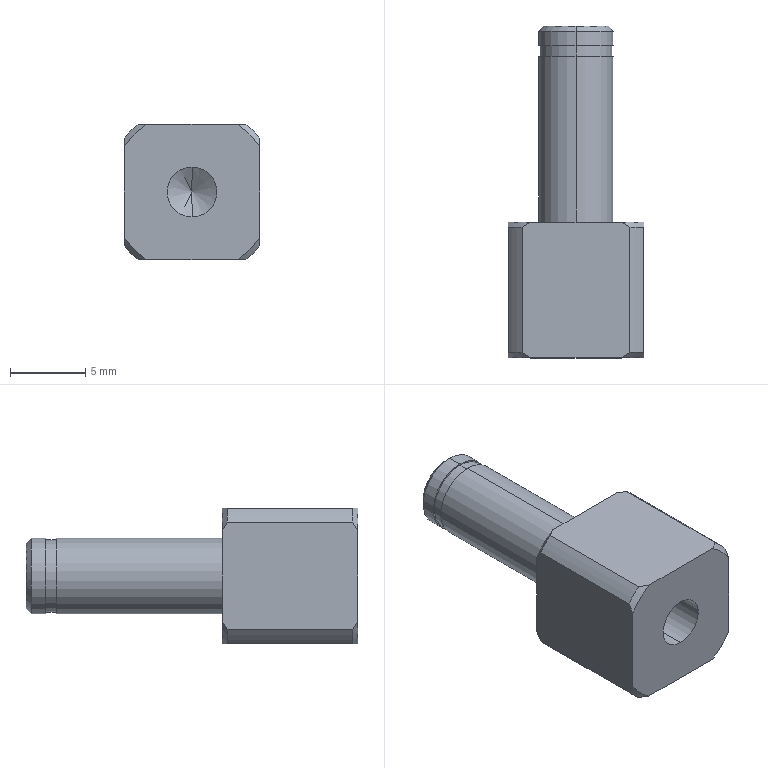Part | NX | features BREP 1 | 1 solid | 33 faces | box 9 x 22 x 9 mm | volume 886.729 mm3 | cylinder 12 | cone 12 | plane 9 | commonest cylinder face diameters 5 x4 11.5 x4 3.3 x2 4.8 x2
STEP:
#1=CARTESIAN_POINT('',(0.,9.1,1.65));
#2=VERTEX_POINT('',#1);
#3=CARTESIAN_POINT('',(0.,0.,1.65));
#4=VERTEX_POINT('',#3);
#5=CARTESIAN_POINT('',(0.,0.,1.65));
#6=DIRECTION('',(0.,-1.,0.));
#7=VECTOR('',#6,1000.);
#8=LINE('',#5,#7);
#9=EDGE_CURVE('',#2,#4,#8,.T.);
#10=ORIENTED_EDGE('',*,*,#9,.F.);
#11=CARTESIAN_POINT('',(0.,9.1,-1.65));
#12=VERTEX_POINT('',#11);
#13=CARTESIAN_POINT('',(0.,9.1,0.));
#14=DIRECTION('',(0.,-1.,0.));
#15=DIRECTION('',(0.,0.,-1.));
#16=AXIS2_PLACEMENT_3D('',#13,#14,#15);
#17=CIRCLE('',#16,1.65);
#18=EDGE_CURVE('',#12,#2,#17,.T.);
#19=ORIENTED_EDGE('',*,*,#18,.F.);
#20=CARTESIAN_POINT('',(0.,0.,-1.65));
#21=VERTEX_POINT('',#20);
#22=CARTESIAN_POINT('',(0.,0.,-1.65));
#23=DIRECTION('',(0.,-1.,0.));
#24=VECTOR('',#23,1000.);
#25=LINE('',#22,#24);
#26=EDGE_CURVE('',#12,#21,#25,.T.);
#27=ORIENTED_EDGE('',*,*,#26,.T.);
#28=CARTESIAN_POINT('',(0.,0.,0.));
#29=DIRECTION('',(0.,-1.,0.));
#30=DIRECTION('',(0.,0.,-1.));
#31=AXIS2_PLACEMENT_3D('',#28,#29,#30);
#32=CIRCLE('',#31,1.65);
#33=EDGE_CURVE('',#21,#4,#32,.T.);
#34=ORIENTED_EDGE('',*,*,#33,.T.);
#35=EDGE_LOOP('',(#10,#19,#27,#34));
#36=FACE_BOUND('',#35,.T.);
#37=CARTESIAN_POINT('',(0.,0.,0.));
#38=DIRECTION('',(0.,-1.,0.));
#39=DIRECTION('',(0.,0.,-1.));
#40=AXIS2_PLACEMENT_3D('',#37,#38,#39);
#41=CYLINDRICAL_SURFACE('',#40,1.65);
#42=ADVANCED_FACE('',(#36),#41,.F.);
#43=CARTESIAN_POINT('',(0.,10.091,0.));
#44=VERTEX_POINT('',#43);
#45=CARTESIAN_POINT('',(0.,9.1,1.65));
#46=DIRECTION('',(0.,-0.515,0.8572));
#47=VECTOR('',#46,1000.);
#48=LINE('',#45,#47);
#49=EDGE_CURVE('',#2,#44,#48,.F.);
#50=ORIENTED_EDGE('',*,*,#49,.T.);
#51=CARTESIAN_POINT('',(0.,9.1,-1.65));
#52=DIRECTION('',(0.,-0.515,-0.8572));
#53=VECTOR('',#52,1000.);
#54=LINE('',#51,#53);
#55=EDGE_CURVE('',#12,#44,#54,.F.);
#56=ORIENTED_EDGE('',*,*,#55,.F.);
#57=ORIENTED_EDGE('',*,*,#18,.T.);
#58=EDGE_LOOP('',(#50,#56,#57));
#59=FACE_BOUND('',#58,.T.);
#60=CARTESIAN_POINT('',(0.,9.1,0.));
#61=DIRECTION('',(0.,-1.,0.));
#62=DIRECTION('',(0.,0.,-1.));
#63=AXIS2_PLACEMENT_3D('',#60,#61,#62);
#64=CONICAL_SURFACE('',#63,1.65,1.03);
#65=ADVANCED_FACE('',(#59),#64,.F.);
#66=CARTESIAN_POINT('',(4.5,0.,2.985));
#67=VERTEX_POINT('',#66);
#68=CARTESIAN_POINT('',(4.5,0.,-2.985));
#69=VERTEX_POINT('',#68);
#70=CARTESIAN_POINT('',(4.5,0.,4.5));
#71=DIRECTION('',(0.,0.,-1.));
#72=VECTOR('',#71,1000.);
#73=LINE('',#70,#72);
#74=EDGE_CURVE('',#67,#69,#73,.T.);
#75=ORIENTED_EDGE('',*,*,#74,.T.);
#76=CARTESIAN_POINT('',(4.5,0.35,-3.579));
#77=VERTEX_POINT('',#76);
#78=CARTESIAN_POINT('',(4.5,0.35,-3.579));
#79=CARTESIAN_POINT('',(4.5,0.2287,-3.385));
#80=CARTESIAN_POINT('',(4.5,0.1115,-3.187));
#81=CARTESIAN_POINT('',(4.5,0.,-2.985));
#82=B_SPLINE_CURVE_WITH_KNOTS('',3,(#78,#79,#80,#81),.UNSPECIFIED.,.F.,.F.,(4,4),(0.008155,0.008844),.UNSPECIFIED.);
#83=EDGE_CURVE('',#77,#69,#82,.T.);
#84=ORIENTED_EDGE('',*,*,#83,.F.);
#85=CARTESIAN_POINT('',(4.5,8.65,-3.579));
#86=VERTEX_POINT('',#85);
#87=CARTESIAN_POINT('',(4.5,0.,-3.579));
#88=DIRECTION('',(0.,1.,0.));
#89=VECTOR('',#88,1000.);
#90=LINE('',#87,#89);
#91=EDGE_CURVE('',#77,#86,#90,.T.);
#92=ORIENTED_EDGE('',*,*,#91,.T.);
#93=CARTESIAN_POINT('',(4.5,9.,-2.985));
#94=VERTEX_POINT('',#93);
#95=CARTESIAN_POINT('',(4.5,9.,-2.985));
#96=CARTESIAN_POINT('',(4.5,8.889,-3.186));
#97=CARTESIAN_POINT('',(4.5,8.771,-3.384));
#98=CARTESIAN_POINT('',(4.5,8.65,-3.579));
#99=B_SPLINE_CURVE_WITH_KNOTS('',3,(#95,#96,#97,#98),.UNSPECIFIED.,.F.,.F.,(4,4),(0.01515,0.01585),.UNSPECIFIED.);
#100=EDGE_CURVE('',#94,#86,#99,.T.);
#101=ORIENTED_EDGE('',*,*,#100,.F.);
#102=CARTESIAN_POINT('',(4.5,9.,2.985));
#103=VERTEX_POINT('',#102);
#104=CARTESIAN_POINT('',(4.5,9.,4.5));
#105=DIRECTION('',(0.,0.,-1.));
#106=VECTOR('',#105,1000.);
#107=LINE('',#104,#106);
#108=EDGE_CURVE('',#103,#94,#107,.T.);
#109=ORIENTED_EDGE('',*,*,#108,.F.);
#110=CARTESIAN_POINT('',(4.5,8.65,3.579));
#111=VERTEX_POINT('',#110);
#112=CARTESIAN_POINT('',(4.5,8.65,3.579));
#113=CARTESIAN_POINT('',(4.5,8.771,3.385));
#114=CARTESIAN_POINT('',(4.5,8.889,3.187));
#115=CARTESIAN_POINT('',(4.5,9.,2.985));
#116=B_SPLINE_CURVE_WITH_KNOTS('',3,(#112,#113,#114,#115),.UNSPECIFIED.,.F.,.F.,(4,4),(0.008155,0.008844),.UNSPECIFIED.);
#117=EDGE_CURVE('',#111,#103,#116,.T.);
#118=ORIENTED_EDGE('',*,*,#117,.F.);
#119=CARTESIAN_POINT('',(4.5,0.35,3.579));
#120=VERTEX_POINT('',#119);
#121=CARTESIAN_POINT('',(4.5,0.,3.579));
#122=DIRECTION('',(0.,-1.,0.));
#123=VECTOR('',#122,1000.);
#124=LINE('',#121,#123);
#125=EDGE_CURVE('',#111,#120,#124,.T.);
#126=ORIENTED_EDGE('',*,*,#125,.T.);
#127=CARTESIAN_POINT('',(4.5,0.,2.985));
#128=CARTESIAN_POINT('',(4.5,0.1114,3.186));
#129=CARTESIAN_POINT('',(4.5,0.2285,3.384));
#130=CARTESIAN_POINT('',(4.5,0.35,3.579));
#131=B_SPLINE_CURVE_WITH_KNOTS('',3,(#127,#128,#129,#130),.UNSPECIFIED.,.F.,.F.,(4,4),(0.01515,0.01585),.UNSPECIFIED.);
#132=EDGE_CURVE('',#67,#120,#131,.T.);
#133=ORIENTED_EDGE('',*,*,#132,.F.);
#134=EDGE_LOOP('',(#75,#84,#92,#101,#109,#118,#126,#133));
#135=FACE_BOUND('',#134,.T.);
#136=CARTESIAN_POINT('',(4.5,0.,4.5));
#137=DIRECTION('',(1.,0.,0.));
#138=DIRECTION('',(0.,0.,-1.));
#139=AXIS2_PLACEMENT_3D('',#136,#137,#138);
#140=PLANE('',#139);
#141=ADVANCED_FACE('',(#135),#140,.T.);
#142=CARTESIAN_POINT('',(-2.985,0.,4.5));
#143=VERTEX_POINT('',#142);
#144=CARTESIAN_POINT('',(2.985,0.,4.5));
#145=VERTEX_POINT('',#144);
#146=CARTESIAN_POINT('',(-4.5,0.,4.5));
#147=DIRECTION('',(1.,0.,0.));
#148=VECTOR('',#147,1000.);
#149=LINE('',#146,#148);
#150=EDGE_CURVE('',#143,#145,#149,.T.);
#151=ORIENTED_EDGE('',*,*,#150,.T.);
#152=CARTESIAN_POINT('',(3.579,0.35,4.5));
#153=VERTEX_POINT('',#152);
#154=CARTESIAN_POINT('',(3.579,0.35,4.5));
#155=CARTESIAN_POINT('',(3.385,0.2287,4.5));
#156=CARTESIAN_POINT('',(3.187,0.1115,4.5));
#157=CARTESIAN_POINT('',(2.985,0.,4.5));
#158=B_SPLINE_CURVE_WITH_KNOTS('',3,(#154,#155,#156,#157),.UNSPECIFIED.,.F.,.F.,(4,4),(0.008155,0.008844),.UNSPECIFIED.);
#159=EDGE_CURVE('',#153,#145,#158,.T.);
#160=ORIENTED_EDGE('',*,*,#159,.F.);
#161=CARTESIAN_POINT('',(3.579,8.65,4.5));
#162=VERTEX_POINT('',#161);
#163=CARTESIAN_POINT('',(3.579,0.,4.5));
#164=DIRECTION('',(0.,1.,0.));
#165=VECTOR('',#164,1000.);
#166=LINE('',#163,#165);
#167=EDGE_CURVE('',#153,#162,#166,.T.);
#168=ORIENTED_EDGE('',*,*,#167,.T.);
#169=CARTESIAN_POINT('',(2.985,9.,4.5));
#170=VERTEX_POINT('',#169);
#171=CARTESIAN_POINT('',(2.985,9.,4.5));
#172=CARTESIAN_POINT('',(3.186,8.889,4.5));
#173=CARTESIAN_POINT('',(3.384,8.771,4.5));
#174=CARTESIAN_POINT('',(3.579,8.65,4.5));
#175=B_SPLINE_CURVE_WITH_KNOTS('',3,(#171,#172,#173,#174),.UNSPECIFIED.,.F.,.F.,(4,4),(0.01515,0.01585),.UNSPECIFIED.);
#176=EDGE_CURVE('',#170,#162,#175,.T.);
#177=ORIENTED_EDGE('',*,*,#176,.F.);
#178=CARTESIAN_POINT('',(-2.985,9.,4.5));
#179=VERTEX_POINT('',#178);
#180=CARTESIAN_POINT('',(-4.5,9.,4.5));
#181=DIRECTION('',(1.,0.,0.));
#182=VECTOR('',#181,1000.);
#183=LINE('',#180,#182);
#184=EDGE_CURVE('',#179,#170,#183,.T.);
#185=ORIENTED_EDGE('',*,*,#184,.F.);
#186=CARTESIAN_POINT('',(-3.579,8.65,4.5));
#187=VERTEX_POINT('',#186);
#188=CARTESIAN_POINT('',(-3.579,8.65,4.5));
#189=CARTESIAN_POINT('',(-3.385,8.771,4.5));
#190=CARTESIAN_POINT('',(-3.187,8.889,4.5));
#191=CARTESIAN_POINT('',(-2.985,9.,4.5));
#192=B_SPLINE_CURVE_WITH_KNOTS('',3,(#188,#189,#190,#191),.UNSPECIFIED.,.F.,.F.,(4,4),(0.008155,0.008844),.UNSPECIFIED.);
#193=EDGE_CURVE('',#187,#179,#192,.T.);
#194=ORIENTED_EDGE('',*,*,#193,.F.);
#195=CARTESIAN_POINT('',(-3.579,0.35,4.5));
#196=VERTEX_POINT('',#195);
#197=CARTESIAN_POINT('',(-3.579,0.,4.5));
#198=DIRECTION('',(0.,-1.,0.));
#199=VECTOR('',#198,1000.);
#200=LINE('',#197,#199);
#201=EDGE_CURVE('',#187,#196,#200,.T.);
#202=ORIENTED_EDGE('',*,*,#201,.T.);
#203=CARTESIAN_POINT('',(-2.985,0.,4.5));
#204=CARTESIAN_POINT('',(-3.186,0.1114,4.5));
#205=CARTESIAN_POINT('',(-3.384,0.2285,4.5));
#206=CARTESIAN_POINT('',(-3.579,0.35,4.5));
#207=B_SPLINE_CURVE_WITH_KNOTS('',3,(#203,#204,#205,#206),.UNSPECIFIED.,.F.,.F.,(4,4),(0.01515,0.01585),.UNSPECIFIED.);
#208=EDGE_CURVE('',#143,#196,#207,.T.);
#209=ORIENTED_EDGE('',*,*,#208,.F.);
#210=EDGE_LOOP('',(#151,#160,#168,#177,#185,#194,#202,#209));
#211=FACE_BOUND('',#210,.T.);
#212=CARTESIAN_POINT('',(-4.5,0.,4.5));
#213=DIRECTION('',(0.,0.,1.));
#214=DIRECTION('',(1.,0.,0.));
#215=AXIS2_PLACEMENT_3D('',#212,#213,#214);
#216=PLANE('',#215);
#217=ADVANCED_FACE('',(#211),#216,.T.);
#218=CARTESIAN_POINT('',(-4.5,0.,-2.985));
#219=VERTEX_POINT('',#218);
#220=CARTESIAN_POINT('',(-4.5,0.,2.985));
#221=VERTEX_POINT('',#220);
#222=CARTESIAN_POINT('',(-4.5,0.,4.5));
#223=DIRECTION('',(0.,0.,1.));
#224=VECTOR('',#223,1000.);
#225=LINE('',#222,#224);
#226=EDGE_CURVE('',#219,#221,#225,.T.);
#227=ORIENTED_EDGE('',*,*,#226,.T.);
#228=CARTESIAN_POINT('',(-4.5,0.35,3.579));
#229=VERTEX_POINT('',#228);
#230=CARTESIAN_POINT('',(-4.5,0.35,3.579));
#231=CARTESIAN_POINT('',(-4.5,0.2287,3.385));
#232=CARTESIAN_POINT('',(-4.5,0.1115,3.187));
#233=CARTESIAN_POINT('',(-4.5,0.,2.985));
#234=B_SPLINE_CURVE_WITH_KNOTS('',3,(#230,#231,#232,#233),.UNSPECIFIED.,.F.,.F.,(4,4),(0.008155,0.008844),.UNSPECIFIED.);
#235=EDGE_CURVE('',#229,#221,#234,.T.);
#236=ORIENTED_EDGE('',*,*,#235,.F.);
#237=CARTESIAN_POINT('',(-4.5,8.65,3.579));
#238=VERTEX_POINT('',#237);
#239=CARTESIAN_POINT('',(-4.5,0.,3.579));
#240=DIRECTION('',(0.,1.,0.));
#241=VECTOR('',#240,1000.);
#242=LINE('',#239,#241);
#243=EDGE_CURVE('',#229,#238,#242,.T.);
#244=ORIENTED_EDGE('',*,*,#243,.T.);
#245=CARTESIAN_POINT('',(-4.5,9.,2.985));
#246=VERTEX_POINT('',#245);
#247=CARTESIAN_POINT('',(-4.5,9.,2.985));
#248=CARTESIAN_POINT('',(-4.5,8.889,3.186));
#249=CARTESIAN_POINT('',(-4.5,8.771,3.384));
#250=CARTESIAN_POINT('',(-4.5,8.65,3.579));
#251=B_SPLINE_CURVE_WITH_KNOTS('',3,(#247,#248,#249,#250),.UNSPECIFIED.,.F.,.F.,(4,4),(0.01515,0.01585),.UNSPECIFIED.);
#252=EDGE_CURVE('',#246,#238,#251,.T.);
#253=ORIENTED_EDGE('',*,*,#252,.F.);
#254=CARTESIAN_POINT('',(-4.5,9.,-2.985));
#255=VERTEX_POINT('',#254);
#256=CARTESIAN_POINT('',(-4.5,9.,4.5));
#257=DIRECTION('',(0.,0.,1.));
#258=VECTOR('',#257,1000.);
#259=LINE('',#256,#258);
#260=EDGE_CURVE('',#255,#246,#259,.T.);
#261=ORIENTED_EDGE('',*,*,#260,.F.);
#262=CARTESIAN_POINT('',(-4.5,8.65,-3.579));
#263=VERTEX_POINT('',#262);
#264=CARTESIAN_POINT('',(-4.5,8.65,-3.579));
#265=CARTESIAN_POINT('',(-4.5,8.771,-3.385));
#266=CARTESIAN_POINT('',(-4.5,8.889,-3.187));
#267=CARTESIAN_POINT('',(-4.5,9.,-2.985));
#268=B_SPLINE_CURVE_WITH_KNOTS('',3,(#264,#265,#266,#267),.UNSPECIFIED.,.F.,.F.,(4,4),(0.008155,0.008844),.UNSPECIFIED.);
#269=EDGE_CURVE('',#263,#255,#268,.T.);
#270=ORIENTED_EDGE('',*,*,#269,.F.);
#271=CARTESIAN_POINT('',(-4.5,0.35,-3.579));
#272=VERTEX_POINT('',#271);
#273=CARTESIAN_POINT('',(-4.5,0.,-3.579));
#274=DIRECTION('',(0.,-1.,0.));
#275=VECTOR('',#274,1000.);
#276=LINE('',#273,#275);
#277=EDGE_CURVE('',#263,#272,#276,.T.);
#278=ORIENTED_EDGE('',*,*,#277,.T.);
#279=CARTESIAN_POINT('',(-4.5,0.,-2.985));
#280=CARTESIAN_POINT('',(-4.5,0.1114,-3.186));
#281=CARTESIAN_POINT('',(-4.5,0.2285,-3.384));
#282=CARTESIAN_POINT('',(-4.5,0.35,-3.579));
#283=B_SPLINE_CURVE_WITH_KNOTS('',3,(#279,#280,#281,#282),.UNSPECIFIED.,.F.,.F.,(4,4),(0.01515,0.01585),.UNSPECIFIED.);
#284=EDGE_CURVE('',#219,#272,#283,.T.);
#285=ORIENTED_EDGE('',*,*,#284,.F.);
#286=EDGE_LOOP('',(#227,#236,#244,#253,#261,#270,#278,#285));
#287=FACE_BOUND('',#286,.T.);
#288=CARTESIAN_POINT('',(-4.5,0.,4.5));
#289=DIRECTION('',(-1.,0.,0.));
#290=DIRECTION('',(0.,0.,1.));
#291=AXIS2_PLACEMENT_3D('',#288,#289,#290);
#292=PLANE('',#291);
#293=ADVANCED_FACE('',(#287),#292,.T.);
#294=CARTESIAN_POINT('',(2.985,0.,-4.5));
#295=VERTEX_POINT('',#294);
#296=CARTESIAN_POINT('',(-2.985,0.,-4.5));
#297=VERTEX_POINT('',#296);
#298=CARTESIAN_POINT('',(-4.5,0.,-4.5));
#299=DIRECTION('',(-1.,0.,0.));
#300=VECTOR('',#299,1000.);
#301=LINE('',#298,#300);
#302=EDGE_CURVE('',#295,#297,#301,.T.);
#303=ORIENTED_EDGE('',*,*,#302,.T.);
#304=CARTESIAN_POINT('',(-3.579,0.35,-4.5));
#305=VERTEX_POINT('',#304);
#306=CARTESIAN_POINT('',(-3.579,0.35,-4.5));
#307=CARTESIAN_POINT('',(-3.385,0.2287,-4.5));
#308=CARTESIAN_POINT('',(-3.187,0.1115,-4.5));
#309=CARTESIAN_POINT('',(-2.985,0.,-4.5));
#310=B_SPLINE_CURVE_WITH_KNOTS('',3,(#306,#307,#308,#309),.UNSPECIFIED.,.F.,.F.,(4,4),(0.008155,0.008844),.UNSPECIFIED.);
#311=EDGE_CURVE('',#305,#297,#310,.T.);
#312=ORIENTED_EDGE('',*,*,#311,.F.);
#313=CARTESIAN_POINT('',(-3.579,8.65,-4.5));
#314=VERTEX_POINT('',#313);
#315=CARTESIAN_POINT('',(-3.579,0.,-4.5));
#316=DIRECTION('',(0.,1.,0.));
#317=VECTOR('',#316,1000.);
#318=LINE('',#315,#317);
#319=EDGE_CURVE('',#305,#314,#318,.T.);
#320=ORIENTED_EDGE('',*,*,#319,.T.);
#321=CARTESIAN_POINT('',(-2.985,9.,-4.5));
#322=VERTEX_POINT('',#321);
#323=CARTESIAN_POINT('',(-2.985,9.,-4.5));
#324=CARTESIAN_POINT('',(-3.186,8.889,-4.5));
#325=CARTESIAN_POINT('',(-3.384,8.771,-4.5));
#326=CARTESIAN_POINT('',(-3.579,8.65,-4.5));
#327=B_SPLINE_CURVE_WITH_KNOTS('',3,(#323,#324,#325,#326),.UNSPECIFIED.,.F.,.F.,(4,4),(0.01515,0.01585),.UNSPECIFIED.);
#328=EDGE_CURVE('',#322,#314,#327,.T.);
#329=ORIENTED_EDGE('',*,*,#328,.F.);
#330=CARTESIAN_POINT('',(2.985,9.,-4.5));
#331=VERTEX_POINT('',#330);
#332=CARTESIAN_POINT('',(-4.5,9.,-4.5));
#333=DIRECTION('',(-1.,0.,0.));
#334=VECTOR('',#333,1000.);
#335=LINE('',#332,#334);
#336=EDGE_CURVE('',#331,#322,#335,.T.);
#337=ORIENTED_EDGE('',*,*,#336,.F.);
#338=CARTESIAN_POINT('',(3.579,8.65,-4.5));
#339=VERTEX_POINT('',#338);
#340=CARTESIAN_POINT('',(3.579,8.65,-4.5));
#341=CARTESIAN_POINT('',(3.385,8.771,-4.5));
#342=CARTESIAN_POINT('',(3.187,8.889,-4.5));
#343=CARTESIAN_POINT('',(2.985,9.,-4.5));
#344=B_SPLINE_CURVE_WITH_KNOTS('',3,(#340,#341,#342,#343),.UNSPECIFIED.,.F.,.F.,(4,4),(0.008155,0.008844),.UNSPECIFIED.);
#345=EDGE_CURVE('',#339,#331,#344,.T.);
#346=ORIENTED_EDGE('',*,*,#345,.F.);
#347=CARTESIAN_POINT('',(3.579,0.35,-4.5));
#348=VERTEX_POINT('',#347);
#349=CARTESIAN_POINT('',(3.579,0.,-4.5));
#350=DIRECTION('',(0.,-1.,0.));
#351=VECTOR('',#350,1000.);
#352=LINE('',#349,#351);
#353=EDGE_CURVE('',#339,#348,#352,.T.);
#354=ORIENTED_EDGE('',*,*,#353,.T.);
#355=CARTESIAN_POINT('',(2.985,0.,-4.5));
#356=CARTESIAN_POINT('',(3.186,0.1114,-4.5));
#357=CARTESIAN_POINT('',(3.384,0.2285,-4.5));
#358=CARTESIAN_POINT('',(3.579,0.35,-4.5));
#359=B_SPLINE_CURVE_WITH_KNOTS('',3,(#355,#356,#357,#358),.UNSPECIFIED.,.F.,.F.,(4,4),(0.01515,0.01585),.UNSPECIFIED.);
#360=EDGE_CURVE('',#295,#348,#359,.T.);
#361=ORIENTED_EDGE('',*,*,#360,.F.);
#362=EDGE_LOOP('',(#303,#312,#320,#329,#337,#346,#354,#361));
#363=FACE_BOUND('',#362,.T.);
#364=CARTESIAN_POINT('',(-4.5,0.,-4.5));
#365=DIRECTION('',(0.,0.,-1.));
#366=DIRECTION('',(-1.,0.,0.));
#367=AXIS2_PLACEMENT_3D('',#364,#365,#366);
#368=PLANE('',#367);
#369=ADVANCED_FACE('',(#363),#368,.T.);
#370=CARTESIAN_POINT('',(0.,22.,2.15));
#371=VERTEX_POINT('',#370);
#372=CARTESIAN_POINT('',(0.,21.65,2.5));
#373=VERTEX_POINT('',#372);
#374=CARTESIAN_POINT('',(0.,21.65,2.5));
#375=DIRECTION('',(0.,-0.7071,0.7071));
#376=VECTOR('',#375,1000.);
#377=LINE('',#374,#376);
#378=EDGE_CURVE('',#371,#373,#377,.T.);
#379=ORIENTED_EDGE('',*,*,#378,.F.);
#380=CARTESIAN_POINT('',(0.,22.,-2.15));
#381=VERTEX_POINT('',#380);
#382=CARTESIAN_POINT('',(0.,22.,0.));
#383=DIRECTION('',(0.,1.,0.));
#384=DIRECTION('',(0.,0.,-1.));
#385=AXIS2_PLACEMENT_3D('',#382,#383,#384);
#386=CIRCLE('',#385,2.15);
#387=EDGE_CURVE('',#381,#371,#386,.T.);
#388=ORIENTED_EDGE('',*,*,#387,.F.);
#389=CARTESIAN_POINT('',(0.,21.65,-2.5));
#390=VERTEX_POINT('',#389);
#391=CARTESIAN_POINT('',(0.,21.65,-2.5));
#392=DIRECTION('',(0.,-0.7071,-0.7071));
#393=VECTOR('',#392,1000.);
#394=LINE('',#391,#393);
#395=EDGE_CURVE('',#381,#390,#394,.T.);
#396=ORIENTED_EDGE('',*,*,#395,.T.);
#397=CARTESIAN_POINT('',(0.,21.65,0.));
#398=DIRECTION('',(0.,-1.,0.));
#399=DIRECTION('',(0.,0.,-1.));
#400=AXIS2_PLACEMENT_3D('',#397,#398,#399);
#401=CIRCLE('',#400,2.5);
#402=EDGE_CURVE('',#373,#390,#401,.T.);
#403=ORIENTED_EDGE('',*,*,#402,.F.);
#404=EDGE_LOOP('',(#379,#388,#396,#403));
#405=FACE_BOUND('',#404,.T.);
#406=CARTESIAN_POINT('',(0.,21.65,0.));
#407=DIRECTION('',(0.,-1.,0.));
#408=DIRECTION('',(0.,0.,-1.));
#409=AXIS2_PLACEMENT_3D('',#406,#407,#408);
#410=CONICAL_SURFACE('',#409,2.5,0.7854);
#411=ADVANCED_FACE('',(#405),#410,.T.);
#412=CARTESIAN_POINT('',(0.,20.,2.5));
#413=VERTEX_POINT('',#412);
#414=CARTESIAN_POINT('',(0.,9.,2.5));
#415=VERTEX_POINT('',#414);
#416=CARTESIAN_POINT('',(0.,0.,2.5));
#417=DIRECTION('',(0.,-1.,0.));
#418=VECTOR('',#417,1000.);
#419=LINE('',#416,#418);
#420=EDGE_CURVE('',#413,#415,#419,.T.);
#421=ORIENTED_EDGE('',*,*,#420,.F.);
#422=CARTESIAN_POINT('',(0.,20.,-2.5));
#423=VERTEX_POINT('',#422);
#424=CARTESIAN_POINT('',(0.,20.,0.));
#425=DIRECTION('',(0.,-1.,0.));
#426=DIRECTION('',(0.,0.,-1.));
#427=AXIS2_PLACEMENT_3D('',#424,#425,#426);
#428=CIRCLE('',#427,2.5);
#429=EDGE_CURVE('',#413,#423,#428,.T.);
#430=ORIENTED_EDGE('',*,*,#429,.T.);
#431=CARTESIAN_POINT('',(0.,9.,-2.5));
#432=VERTEX_POINT('',#431);
#433=CARTESIAN_POINT('',(0.,0.,-2.5));
#434=DIRECTION('',(0.,-1.,0.));
#435=VECTOR('',#434,1000.);
#436=LINE('',#433,#435);
#437=EDGE_CURVE('',#423,#432,#436,.T.);
#438=ORIENTED_EDGE('',*,*,#437,.T.);
#439=CARTESIAN_POINT('',(0.,9.,0.));
#440=DIRECTION('',(0.,-1.,0.));
#441=DIRECTION('',(0.,0.,-1.));
#442=AXIS2_PLACEMENT_3D('',#439,#440,#441);
#443=CIRCLE('',#442,2.5);
#444=EDGE_CURVE('',#415,#432,#443,.T.);
#445=ORIENTED_EDGE('',*,*,#444,.F.);
#446=EDGE_LOOP('',(#421,#430,#438,#445));
#447=FACE_BOUND('',#446,.T.);
#448=CARTESIAN_POINT('',(0.,0.,0.));
#449=DIRECTION('',(0.,-1.,0.));
#450=DIRECTION('',(0.,0.,-1.));
#451=AXIS2_PLACEMENT_3D('',#448,#449,#450);
#452=CYLINDRICAL_SURFACE('',#451,2.5);
#453=ADVANCED_FACE('',(#447),#452,.T.);
#454=CARTESIAN_POINT('',(0.,20.,0.));
#455=DIRECTION('',(0.,-1.,0.));
#456=DIRECTION('',(0.,0.,-1.));
#457=AXIS2_PLACEMENT_3D('',#454,#455,#456);
#458=CIRCLE('',#457,2.5);
#459=EDGE_CURVE('',#423,#413,#458,.T.);
#460=ORIENTED_EDGE('',*,*,#459,.F.);
#461=ORIENTED_EDGE('',*,*,#429,.F.);
#462=EDGE_LOOP('',(#460,#461));
#463=FACE_BOUND('',#462,.T.);
#464=CARTESIAN_POINT('',(0.,20.,-2.4));
#465=VERTEX_POINT('',#464);
#466=CARTESIAN_POINT('',(0.,20.,2.4));
#467=VERTEX_POINT('',#466);
#468=CARTESIAN_POINT('',(0.,20.,0.));
#469=DIRECTION('',(0.,-1.,0.));
#470=DIRECTION('',(0.,0.,-1.));
#471=AXIS2_PLACEMENT_3D('',#468,#469,#470);
#472=CIRCLE('',#471,2.4);
#473=EDGE_CURVE('',#465,#467,#472,.T.);
#474=ORIENTED_EDGE('',*,*,#473,.T.);
#475=CARTESIAN_POINT('',(0.,20.,0.));
#476=DIRECTION('',(0.,-1.,0.));
#477=DIRECTION('',(0.,0.,-1.));
#478=AXIS2_PLACEMENT_3D('',#475,#476,#477);
#479=CIRCLE('',#478,2.4);
#480=EDGE_CURVE('',#467,#465,#479,.T.);
#481=ORIENTED_EDGE('',*,*,#480,.T.);
#482=EDGE_LOOP('',(#474,#481));
#483=FACE_BOUND('',#482,.T.);
#484=CARTESIAN_POINT('',(0.,20.,0.));
#485=DIRECTION('',(0.,1.,0.));
#486=DIRECTION('',(0.,0.,1.));
#487=AXIS2_PLACEMENT_3D('',#484,#485,#486);
#488=PLANE('',#487);
#489=ADVANCED_FACE('',(#463,#483),#488,.T.);
#490=CARTESIAN_POINT('',(0.,20.7,2.4));
#491=VERTEX_POINT('',#490);
#492=CARTESIAN_POINT('',(0.,0.,2.4));
#493=DIRECTION('',(0.,-1.,0.));
#494=VECTOR('',#493,1000.);
#495=LINE('',#492,#494);
#496=EDGE_CURVE('',#491,#467,#495,.T.);
#497=ORIENTED_EDGE('',*,*,#496,.F.);
#498=CARTESIAN_POINT('',(0.,20.7,-2.4));
#499=VERTEX_POINT('',#498);
#500=CARTESIAN_POINT('',(0.,20.7,0.));
#501=DIRECTION('',(0.,-1.,0.));
#502=DIRECTION('',(0.,0.,-1.));
#503=AXIS2_PLACEMENT_3D('',#500,#501,#502);
#504=CIRCLE('',#503,2.4);
#505=EDGE_CURVE('',#491,#499,#504,.T.);
#506=ORIENTED_EDGE('',*,*,#505,.T.);
#507=CARTESIAN_POINT('',(0.,0.,-2.4));
#508=DIRECTION('',(0.,-1.,0.));
#509=VECTOR('',#508,1000.);
#510=LINE('',#507,#509);
#511=EDGE_CURVE('',#499,#465,#510,.T.);
#512=ORIENTED_EDGE('',*,*,#511,.T.);
#513=ORIENTED_EDGE('',*,*,#480,.F.);
#514=EDGE_LOOP('',(#497,#506,#512,#513));
#515=FACE_BOUND('',#514,.T.);
#516=CARTESIAN_POINT('',(0.,0.,0.));
#517=DIRECTION('',(0.,-1.,0.));
#518=DIRECTION('',(0.,0.,-1.));
#519=AXIS2_PLACEMENT_3D('',#516,#517,#518);
#520=CYLINDRICAL_SURFACE('',#519,2.4);
#521=ADVANCED_FACE('',(#515),#520,.T.);
#522=CARTESIAN_POINT('',(0.,20.7,-2.5));
#523=VERTEX_POINT('',#522);
#524=CARTESIAN_POINT('',(0.,20.7,2.5));
#525=VERTEX_POINT('',#524);
#526=CARTESIAN_POINT('',(0.,20.7,0.));
#527=DIRECTION('',(0.,-1.,0.));
#528=DIRECTION('',(0.,0.,-1.));
#529=AXIS2_PLACEMENT_3D('',#526,#527,#528);
#530=CIRCLE('',#529,2.5);
#531=EDGE_CURVE('',#523,#525,#530,.T.);
#532=ORIENTED_EDGE('',*,*,#531,.T.);
#533=CARTESIAN_POINT('',(0.,20.7,0.));
#534=DIRECTION('',(0.,-1.,0.));
#535=DIRECTION('',(0.,0.,-1.));
#536=AXIS2_PLACEMENT_3D('',#533,#534,#535);
#537=CIRCLE('',#536,2.5);
#538=EDGE_CURVE('',#525,#523,#537,.T.);
#539=ORIENTED_EDGE('',*,*,#538,.T.);
#540=EDGE_LOOP('',(#532,#539));
#541=FACE_BOUND('',#540,.T.);
#542=CARTESIAN_POINT('',(0.,20.7,0.));
#543=DIRECTION('',(0.,-1.,0.));
#544=DIRECTION('',(0.,0.,-1.));
#545=AXIS2_PLACEMENT_3D('',#542,#543,#544);
#546=CIRCLE('',#545,2.4);
#547=EDGE_CURVE('',#499,#491,#546,.T.);
#548=ORIENTED_EDGE('',*,*,#547,.F.);
#549=ORIENTED_EDGE('',*,*,#505,.F.);
#550=EDGE_LOOP('',(#548,#549));
#551=FACE_BOUND('',#550,.T.);
#552=CARTESIAN_POINT('',(0.,20.7,0.));
#553=DIRECTION('',(0.,1.,0.));
#554=DIRECTION('',(0.,0.,1.));
#555=AXIS2_PLACEMENT_3D('',#552,#553,#554);
#556=PLANE('',#555);
#557=ADVANCED_FACE('',(#541,#551),#556,.F.);
#558=CARTESIAN_POINT('',(0.,0.,2.5));
#559=DIRECTION('',(0.,-1.,0.));
#560=VECTOR('',#559,1000.);
#561=LINE('',#558,#560);
#562=EDGE_CURVE('',#373,#525,#561,.T.);
#563=ORIENTED_EDGE('',*,*,#562,.F.);
#564=ORIENTED_EDGE('',*,*,#402,.T.);
#565=CARTESIAN_POINT('',(0.,0.,-2.5));
#566=DIRECTION('',(0.,-1.,0.));
#567=VECTOR('',#566,1000.);
#568=LINE('',#565,#567);
#569=EDGE_CURVE('',#390,#523,#568,.T.);
#570=ORIENTED_EDGE('',*,*,#569,.T.);
#571=ORIENTED_EDGE('',*,*,#538,.F.);
#572=EDGE_LOOP('',(#563,#564,#570,#571));
#573=FACE_BOUND('',#572,.T.);
#574=CARTESIAN_POINT('',(0.,0.,0.));
#575=DIRECTION('',(0.,-1.,0.));
#576=DIRECTION('',(0.,0.,-1.));
#577=AXIS2_PLACEMENT_3D('',#574,#575,#576);
#578=CYLINDRICAL_SURFACE('',#577,2.5);
#579=ADVANCED_FACE('',(#573),#578,.T.);
#580=ORIENTED_EDGE('',*,*,#387,.T.);
#581=CARTESIAN_POINT('',(0.,22.,0.));
#582=DIRECTION('',(0.,1.,0.));
#583=DIRECTION('',(0.,0.,-1.));
#584=AXIS2_PLACEMENT_3D('',#581,#582,#583);
#585=CIRCLE('',#584,2.15);
#586=EDGE_CURVE('',#371,#381,#585,.T.);
#587=ORIENTED_EDGE('',*,*,#586,.T.);
#588=EDGE_LOOP('',(#580,#587));
#589=FACE_BOUND('',#588,.T.);
#590=CARTESIAN_POINT('',(0.,22.,0.));
#591=DIRECTION('',(0.,-1.,0.));
#592=DIRECTION('',(0.,0.,-1.));
#593=AXIS2_PLACEMENT_3D('',#590,#591,#592);
#594=PLANE('',#593);
#595=ADVANCED_FACE('',(#589),#594,.F.);
#596=CARTESIAN_POINT('',(0.,8.65,0.));
#597=DIRECTION('',(0.,-1.,0.));
#598=DIRECTION('',(0.,0.,-1.));
#599=AXIS2_PLACEMENT_3D('',#596,#597,#598);
#600=CIRCLE('',#599,5.75);
#601=EDGE_CURVE('',#263,#314,#600,.T.);
#602=ORIENTED_EDGE('',*,*,#601,.F.);
#603=ORIENTED_EDGE('',*,*,#269,.T.);
#604=CARTESIAN_POINT('',(0.,9.,0.));
#605=DIRECTION('',(0.,1.,0.));
#606=DIRECTION('',(0.,0.,-1.));
#607=AXIS2_PLACEMENT_3D('',#604,#605,#606);
#608=CIRCLE('',#607,5.4);
#609=EDGE_CURVE('',#322,#255,#608,.T.);
#610=ORIENTED_EDGE('',*,*,#609,.F.);
#611=ORIENTED_EDGE('',*,*,#328,.T.);
#612=EDGE_LOOP('',(#602,#603,#610,#611));
#613=FACE_BOUND('',#612,.T.);
#614=CARTESIAN_POINT('',(0.,8.65,0.));
#615=DIRECTION('',(0.,-1.,0.));
#616=DIRECTION('',(0.,0.,-1.));
#617=AXIS2_PLACEMENT_3D('',#614,#615,#616);
#618=CONICAL_SURFACE('',#617,5.75,0.7854);
#619=ADVANCED_FACE('',(#613),#618,.T.);
#620=CARTESIAN_POINT('',(0.,8.65,0.));
#621=DIRECTION('',(0.,-1.,0.));
#622=DIRECTION('',(0.,0.,-1.));
#623=AXIS2_PLACEMENT_3D('',#620,#621,#622);
#624=CIRCLE('',#623,5.75);
#625=EDGE_CURVE('',#187,#238,#624,.T.);
#626=ORIENTED_EDGE('',*,*,#625,.F.);
#627=ORIENTED_EDGE('',*,*,#193,.T.);
#628=CARTESIAN_POINT('',(0.,9.,0.));
#629=DIRECTION('',(0.,1.,0.));
#630=DIRECTION('',(0.,0.,-1.));
#631=AXIS2_PLACEMENT_3D('',#628,#629,#630);
#632=CIRCLE('',#631,5.4);
#633=EDGE_CURVE('',#246,#179,#632,.T.);
#634=ORIENTED_EDGE('',*,*,#633,.F.);
#635=ORIENTED_EDGE('',*,*,#252,.T.);
#636=EDGE_LOOP('',(#626,#627,#634,#635));
#637=FACE_BOUND('',#636,.T.);
#638=CARTESIAN_POINT('',(0.,8.65,0.));
#639=DIRECTION('',(0.,-1.,0.));
#640=DIRECTION('',(0.,0.,-1.));
#641=AXIS2_PLACEMENT_3D('',#638,#639,#640);
#642=CONICAL_SURFACE('',#641,5.75,0.7854);
#643=ADVANCED_FACE('',(#637),#642,.T.);
#644=CARTESIAN_POINT('',(0.,9.,0.));
#645=DIRECTION('',(0.,1.,0.));
#646=DIRECTION('',(0.,0.,-1.));
#647=AXIS2_PLACEMENT_3D('',#644,#645,#646);
#648=CIRCLE('',#647,5.4);
#649=EDGE_CURVE('',#94,#331,#648,.T.);
#650=ORIENTED_EDGE('',*,*,#649,.F.);
#651=ORIENTED_EDGE('',*,*,#100,.T.);
#652=CARTESIAN_POINT('',(0.,8.65,0.));
#653=DIRECTION('',(0.,-1.,0.));
#654=DIRECTION('',(0.,0.,-1.));
#655=AXIS2_PLACEMENT_3D('',#652,#653,#654);
#656=CIRCLE('',#655,5.75);
#657=EDGE_CURVE('',#339,#86,#656,.T.);
#658=ORIENTED_EDGE('',*,*,#657,.F.);
#659=ORIENTED_EDGE('',*,*,#345,.T.);
#660=EDGE_LOOP('',(#650,#651,#658,#659));
#661=FACE_BOUND('',#660,.T.);
#662=CARTESIAN_POINT('',(0.,8.65,0.));
#663=DIRECTION('',(0.,-1.,0.));
#664=DIRECTION('',(0.,0.,-1.));
#665=AXIS2_PLACEMENT_3D('',#662,#663,#664);
#666=CONICAL_SURFACE('',#665,5.75,0.7854);
#667=ADVANCED_FACE('',(#661),#666,.T.);
#668=CARTESIAN_POINT('',(0.,8.65,0.));
#669=DIRECTION('',(0.,-1.,0.));
#670=DIRECTION('',(0.,0.,-1.));
#671=AXIS2_PLACEMENT_3D('',#668,#669,#670);
#672=CIRCLE('',#671,5.75);
#673=EDGE_CURVE('',#111,#162,#672,.T.);
#674=ORIENTED_EDGE('',*,*,#673,.F.);
#675=ORIENTED_EDGE('',*,*,#117,.T.);
#676=CARTESIAN_POINT('',(0.,9.,0.));
#677=DIRECTION('',(0.,1.,0.));
#678=DIRECTION('',(0.,0.,-1.));
#679=AXIS2_PLACEMENT_3D('',#676,#677,#678);
#680=CIRCLE('',#679,5.4);
#681=EDGE_CURVE('',#170,#103,#680,.T.);
#682=ORIENTED_EDGE('',*,*,#681,.F.);
#683=ORIENTED_EDGE('',*,*,#176,.T.);
#684=EDGE_LOOP('',(#674,#675,#682,#683));
#685=FACE_BOUND('',#684,.T.);
#686=CARTESIAN_POINT('',(0.,8.65,0.));
#687=DIRECTION('',(0.,-1.,0.));
#688=DIRECTION('',(0.,0.,-1.));
#689=AXIS2_PLACEMENT_3D('',#686,#687,#688);
#690=CONICAL_SURFACE('',#689,5.75,0.7854);
#691=ADVANCED_FACE('',(#685),#690,.T.);
#692=CARTESIAN_POINT('',(0.,0.,0.));
#693=DIRECTION('',(0.,-1.,0.));
#694=DIRECTION('',(0.,0.,1.));
#695=AXIS2_PLACEMENT_3D('',#692,#693,#694);
#696=CIRCLE('',#695,5.4);
#697=EDGE_CURVE('',#219,#297,#696,.T.);
#698=ORIENTED_EDGE('',*,*,#697,.F.);
#699=ORIENTED_EDGE('',*,*,#284,.T.);
#700=CARTESIAN_POINT('',(0.,0.35,0.));
#701=DIRECTION('',(0.,1.,0.));
#702=DIRECTION('',(0.,0.,1.));
#703=AXIS2_PLACEMENT_3D('',#700,#701,#702);
#704=CIRCLE('',#703,5.75);
#705=EDGE_CURVE('',#305,#272,#704,.T.);
#706=ORIENTED_EDGE('',*,*,#705,.F.);
#707=ORIENTED_EDGE('',*,*,#311,.T.);
#708=EDGE_LOOP('',(#698,#699,#706,#707));
#709=FACE_BOUND('',#708,.T.);
#710=CARTESIAN_POINT('',(0.,0.,0.));
#711=DIRECTION('',(0.,1.,0.));
#712=DIRECTION('',(0.,0.,1.));
#713=AXIS2_PLACEMENT_3D('',#710,#711,#712);
#714=CONICAL_SURFACE('',#713,5.4,0.7854);
#715=ADVANCED_FACE('',(#709),#714,.T.);
#716=CARTESIAN_POINT('',(0.,0.,0.));
#717=DIRECTION('',(0.,-1.,0.));
#718=DIRECTION('',(0.,0.,1.));
#719=AXIS2_PLACEMENT_3D('',#716,#717,#718);
#720=CIRCLE('',#719,5.4);
#721=EDGE_CURVE('',#143,#221,#720,.T.);
#722=ORIENTED_EDGE('',*,*,#721,.F.);
#723=ORIENTED_EDGE('',*,*,#208,.T.);
#724=CARTESIAN_POINT('',(0.,0.35,0.));
#725=DIRECTION('',(0.,1.,0.));
#726=DIRECTION('',(0.,0.,1.));
#727=AXIS2_PLACEMENT_3D('',#724,#725,#726);
#728=CIRCLE('',#727,5.75);
#729=EDGE_CURVE('',#229,#196,#728,.T.);
#730=ORIENTED_EDGE('',*,*,#729,.F.);
#731=ORIENTED_EDGE('',*,*,#235,.T.);
#732=EDGE_LOOP('',(#722,#723,#730,#731));
#733=FACE_BOUND('',#732,.T.);
#734=CARTESIAN_POINT('',(0.,0.,0.));
#735=DIRECTION('',(0.,1.,0.));
#736=DIRECTION('',(0.,0.,1.));
#737=AXIS2_PLACEMENT_3D('',#734,#735,#736);
#738=CONICAL_SURFACE('',#737,5.4,0.7854);
#739=ADVANCED_FACE('',(#733),#738,.T.);
#740=CARTESIAN_POINT('',(0.,0.,0.));
#741=DIRECTION('',(0.,-1.,0.));
#742=DIRECTION('',(0.,0.,1.));
#743=AXIS2_PLACEMENT_3D('',#740,#741,#742);
#744=CIRCLE('',#743,5.4);
#745=EDGE_CURVE('',#67,#145,#744,.T.);
#746=ORIENTED_EDGE('',*,*,#745,.F.);
#747=ORIENTED_EDGE('',*,*,#132,.T.);
#748=CARTESIAN_POINT('',(0.,0.35,0.));
#749=DIRECTION('',(0.,1.,0.));
#750=DIRECTION('',(0.,0.,1.));
#751=AXIS2_PLACEMENT_3D('',#748,#749,#750);
#752=CIRCLE('',#751,5.75);
#753=EDGE_CURVE('',#153,#120,#752,.T.);
#754=ORIENTED_EDGE('',*,*,#753,.F.);
#755=ORIENTED_EDGE('',*,*,#159,.T.);
#756=EDGE_LOOP('',(#746,#747,#754,#755));
#757=FACE_BOUND('',#756,.T.);
#758=CARTESIAN_POINT('',(0.,0.,0.));
#759=DIRECTION('',(0.,1.,0.));
#760=DIRECTION('',(0.,0.,1.));
#761=AXIS2_PLACEMENT_3D('',#758,#759,#760);
#762=CONICAL_SURFACE('',#761,5.4,0.7854);
#763=ADVANCED_FACE('',(#757),#762,.T.);
#764=CARTESIAN_POINT('',(0.,0.35,0.));
#765=DIRECTION('',(0.,1.,0.));
#766=DIRECTION('',(0.,0.,1.));
#767=AXIS2_PLACEMENT_3D('',#764,#765,#766);
#768=CIRCLE('',#767,5.75);
#769=EDGE_CURVE('',#77,#348,#768,.T.);
#770=ORIENTED_EDGE('',*,*,#769,.F.);
#771=ORIENTED_EDGE('',*,*,#83,.T.);
#772=CARTESIAN_POINT('',(0.,0.,0.));
#773=DIRECTION('',(0.,-1.,0.));
#774=DIRECTION('',(0.,0.,1.));
#775=AXIS2_PLACEMENT_3D('',#772,#773,#774);
#776=CIRCLE('',#775,5.4);
#777=EDGE_CURVE('',#295,#69,#776,.T.);
#778=ORIENTED_EDGE('',*,*,#777,.F.);
#779=ORIENTED_EDGE('',*,*,#360,.T.);
#780=EDGE_LOOP('',(#770,#771,#778,#779));
#781=FACE_BOUND('',#780,.T.);
#782=CARTESIAN_POINT('',(0.,0.,0.));
#783=DIRECTION('',(0.,1.,0.));
#784=DIRECTION('',(0.,0.,1.));
#785=AXIS2_PLACEMENT_3D('',#782,#783,#784);
#786=CONICAL_SURFACE('',#785,5.4,0.7854);
#787=ADVANCED_FACE('',(#781),#786,.T.);
#788=ORIENTED_EDGE('',*,*,#277,.F.);
#789=ORIENTED_EDGE('',*,*,#601,.T.);
#790=ORIENTED_EDGE('',*,*,#319,.F.);
#791=ORIENTED_EDGE('',*,*,#705,.T.);
#792=EDGE_LOOP('',(#788,#789,#790,#791));
#793=FACE_BOUND('',#792,.T.);
#794=CARTESIAN_POINT('',(0.,0.,0.));
#795=DIRECTION('',(0.,-1.,0.));
#796=DIRECTION('',(0.,0.,-1.));
#797=AXIS2_PLACEMENT_3D('',#794,#795,#796);
#798=CYLINDRICAL_SURFACE('',#797,5.75);
#799=ADVANCED_FACE('',(#793),#798,.T.);
#800=ORIENTED_EDGE('',*,*,#201,.F.);
#801=ORIENTED_EDGE('',*,*,#625,.T.);
#802=ORIENTED_EDGE('',*,*,#243,.F.);
#803=ORIENTED_EDGE('',*,*,#729,.T.);
#804=EDGE_LOOP('',(#800,#801,#802,#803));
#805=FACE_BOUND('',#804,.T.);
#806=CARTESIAN_POINT('',(0.,0.,0.));
#807=DIRECTION('',(0.,-1.,0.));
#808=DIRECTION('',(0.,0.,-1.));
#809=AXIS2_PLACEMENT_3D('',#806,#807,#808);
#810=CYLINDRICAL_SURFACE('',#809,5.75);
#811=ADVANCED_FACE('',(#805),#810,.T.);
#812=ORIENTED_EDGE('',*,*,#91,.F.);
#813=ORIENTED_EDGE('',*,*,#769,.T.);
#814=ORIENTED_EDGE('',*,*,#353,.F.);
#815=ORIENTED_EDGE('',*,*,#657,.T.);
#816=EDGE_LOOP('',(#812,#813,#814,#815));
#817=FACE_BOUND('',#816,.T.);
#818=CARTESIAN_POINT('',(0.,0.,0.));
#819=DIRECTION('',(0.,-1.,0.));
#820=DIRECTION('',(0.,0.,-1.));
#821=AXIS2_PLACEMENT_3D('',#818,#819,#820);
#822=CYLINDRICAL_SURFACE('',#821,5.75);
#823=ADVANCED_FACE('',(#817),#822,.T.);
#824=ORIENTED_EDGE('',*,*,#125,.F.);
#825=ORIENTED_EDGE('',*,*,#673,.T.);
#826=ORIENTED_EDGE('',*,*,#167,.F.);
#827=ORIENTED_EDGE('',*,*,#753,.T.);
#828=EDGE_LOOP('',(#824,#825,#826,#827));
#829=FACE_BOUND('',#828,.T.);
#830=CARTESIAN_POINT('',(0.,0.,0.));
#831=DIRECTION('',(0.,-1.,0.));
#832=DIRECTION('',(0.,0.,-1.));
#833=AXIS2_PLACEMENT_3D('',#830,#831,#832);
#834=CYLINDRICAL_SURFACE('',#833,5.75);
#835=ADVANCED_FACE('',(#829),#834,.T.);
#836=ORIENTED_EDGE('',*,*,#108,.T.);
#837=ORIENTED_EDGE('',*,*,#649,.T.);
#838=ORIENTED_EDGE('',*,*,#336,.T.);
#839=ORIENTED_EDGE('',*,*,#609,.T.);
#840=ORIENTED_EDGE('',*,*,#260,.T.);
#841=ORIENTED_EDGE('',*,*,#633,.T.);
#842=ORIENTED_EDGE('',*,*,#184,.T.);
#843=ORIENTED_EDGE('',*,*,#681,.T.);
#844=EDGE_LOOP('',(#836,#837,#838,#839,#840,#841,#842,#843));
#845=FACE_BOUND('',#844,.T.);
#846=CARTESIAN_POINT('',(0.,9.,0.));
#847=DIRECTION('',(0.,-1.,0.));
#848=DIRECTION('',(0.,0.,-1.));
#849=AXIS2_PLACEMENT_3D('',#846,#847,#848);
#850=CIRCLE('',#849,2.5);
#851=EDGE_CURVE('',#432,#415,#850,.T.);
#852=ORIENTED_EDGE('',*,*,#851,.T.);
#853=ORIENTED_EDGE('',*,*,#444,.T.);
#854=EDGE_LOOP('',(#852,#853));
#855=FACE_BOUND('',#854,.T.);
#856=CARTESIAN_POINT('',(0.,9.,0.));
#857=DIRECTION('',(0.,-1.,0.));
#858=DIRECTION('',(0.,0.,-1.));
#859=AXIS2_PLACEMENT_3D('',#856,#857,#858);
#860=PLANE('',#859);
#861=ADVANCED_FACE('',(#845,#855),#860,.F.);
#862=ORIENTED_EDGE('',*,*,#33,.F.);
#863=CARTESIAN_POINT('',(0.,0.,0.));
#864=DIRECTION('',(0.,-1.,0.));
#865=DIRECTION('',(0.,0.,-1.));
#866=AXIS2_PLACEMENT_3D('',#863,#864,#865);
#867=CIRCLE('',#866,1.65);
#868=EDGE_CURVE('',#4,#21,#867,.T.);
#869=ORIENTED_EDGE('',*,*,#868,.F.);
#870=EDGE_LOOP('',(#862,#869));
#871=FACE_BOUND('',#870,.T.);
#872=ORIENTED_EDGE('',*,*,#74,.F.);
#873=ORIENTED_EDGE('',*,*,#745,.T.);
#874=ORIENTED_EDGE('',*,*,#150,.F.);
#875=ORIENTED_EDGE('',*,*,#721,.T.);
#876=ORIENTED_EDGE('',*,*,#226,.F.);
#877=ORIENTED_EDGE('',*,*,#697,.T.);
#878=ORIENTED_EDGE('',*,*,#302,.F.);
#879=ORIENTED_EDGE('',*,*,#777,.T.);
#880=EDGE_LOOP('',(#872,#873,#874,#875,#876,#877,#878,#879));
#881=FACE_BOUND('',#880,.T.);
#882=CARTESIAN_POINT('',(0.,0.,0.));
#883=DIRECTION('',(0.,1.,0.));
#884=DIRECTION('',(0.,0.,1.));
#885=AXIS2_PLACEMENT_3D('',#882,#883,#884);
#886=PLANE('',#885);
#887=ADVANCED_FACE('',(#871,#881),#886,.F.);
#888=CARTESIAN_POINT('',(0.,21.65,0.));
#889=DIRECTION('',(0.,-1.,0.));
#890=DIRECTION('',(0.,0.,-1.));
#891=AXIS2_PLACEMENT_3D('',#888,#889,#890);
#892=CIRCLE('',#891,2.5);
#893=EDGE_CURVE('',#390,#373,#892,.T.);
#894=ORIENTED_EDGE('',*,*,#893,.T.);
#895=ORIENTED_EDGE('',*,*,#562,.T.);
#896=ORIENTED_EDGE('',*,*,#531,.F.);
#897=ORIENTED_EDGE('',*,*,#569,.F.);
#898=EDGE_LOOP('',(#894,#895,#896,#897));
#899=FACE_BOUND('',#898,.T.);
#900=CARTESIAN_POINT('',(0.,0.,0.));
#901=DIRECTION('',(0.,-1.,0.));
#902=DIRECTION('',(0.,0.,-1.));
#903=AXIS2_PLACEMENT_3D('',#900,#901,#902);
#904=CYLINDRICAL_SURFACE('',#903,2.5);
#905=ADVANCED_FACE('',(#899),#904,.T.);
#906=ORIENTED_EDGE('',*,*,#547,.T.);
#907=ORIENTED_EDGE('',*,*,#496,.T.);
#908=ORIENTED_EDGE('',*,*,#473,.F.);
#909=ORIENTED_EDGE('',*,*,#511,.F.);
#910=EDGE_LOOP('',(#906,#907,#908,#909));
#911=FACE_BOUND('',#910,.T.);
#912=CARTESIAN_POINT('',(0.,0.,0.));
#913=DIRECTION('',(0.,-1.,0.));
#914=DIRECTION('',(0.,0.,-1.));
#915=AXIS2_PLACEMENT_3D('',#912,#913,#914);
#916=CYLINDRICAL_SURFACE('',#915,2.4);
#917=ADVANCED_FACE('',(#911),#916,.T.);
#918=ORIENTED_EDGE('',*,*,#459,.T.);
#919=ORIENTED_EDGE('',*,*,#420,.T.);
#920=ORIENTED_EDGE('',*,*,#851,.F.);
#921=ORIENTED_EDGE('',*,*,#437,.F.);
#922=EDGE_LOOP('',(#918,#919,#920,#921));
#923=FACE_BOUND('',#922,.T.);
#924=CARTESIAN_POINT('',(0.,0.,0.));
#925=DIRECTION('',(0.,-1.,0.));
#926=DIRECTION('',(0.,0.,-1.));
#927=AXIS2_PLACEMENT_3D('',#924,#925,#926);
#928=CYLINDRICAL_SURFACE('',#927,2.5);
#929=ADVANCED_FACE('',(#923),#928,.T.);
#930=ORIENTED_EDGE('',*,*,#586,.F.);
#931=ORIENTED_EDGE('',*,*,#378,.T.);
#932=ORIENTED_EDGE('',*,*,#893,.F.);
#933=ORIENTED_EDGE('',*,*,#395,.F.);
#934=EDGE_LOOP('',(#930,#931,#932,#933));
#935=FACE_BOUND('',#934,.T.);
#936=CARTESIAN_POINT('',(0.,21.65,0.));
#937=DIRECTION('',(0.,-1.,0.));
#938=DIRECTION('',(0.,0.,-1.));
#939=AXIS2_PLACEMENT_3D('',#936,#937,#938);
#940=CONICAL_SURFACE('',#939,2.5,0.7854);
#941=ADVANCED_FACE('',(#935),#940,.T.);
#942=ORIENTED_EDGE('',*,*,#55,.T.);
#943=ORIENTED_EDGE('',*,*,#49,.F.);
#944=CARTESIAN_POINT('',(0.,9.1,0.));
#945=DIRECTION('',(0.,-1.,0.));
#946=DIRECTION('',(0.,0.,-1.));
#947=AXIS2_PLACEMENT_3D('',#944,#945,#946);
#948=CIRCLE('',#947,1.65);
#949=EDGE_CURVE('',#2,#12,#948,.T.);
#950=ORIENTED_EDGE('',*,*,#949,.T.);
#951=EDGE_LOOP('',(#942,#943,#950));
#952=FACE_BOUND('',#951,.T.);
#953=CARTESIAN_POINT('',(0.,9.1,0.));
#954=DIRECTION('',(0.,-1.,0.));
#955=DIRECTION('',(0.,0.,-1.));
#956=AXIS2_PLACEMENT_3D('',#953,#954,#955);
#957=CONICAL_SURFACE('',#956,1.65,1.03);
#958=ADVANCED_FACE('',(#952),#957,.F.);
#959=ORIENTED_EDGE('',*,*,#949,.F.);
#960=ORIENTED_EDGE('',*,*,#9,.T.);
#961=ORIENTED_EDGE('',*,*,#868,.T.);
#962=ORIENTED_EDGE('',*,*,#26,.F.);
#963=EDGE_LOOP('',(#959,#960,#961,#962));
#964=FACE_BOUND('',#963,.T.);
#965=CARTESIAN_POINT('',(0.,0.,0.));
#966=DIRECTION('',(0.,-1.,0.));
#967=DIRECTION('',(0.,0.,-1.));
#968=AXIS2_PLACEMENT_3D('',#965,#966,#967);
#969=CYLINDRICAL_SURFACE('',#968,1.65);
#970=ADVANCED_FACE('',(#964),#969,.F.);
#971=CLOSED_SHELL('',(#42,#65,#141,#217,#293,#369,#411,#453,#489,#521,#557,#579,#595,#619,#643,#667,#691,#715,#739,#763,#787,#799,#811,#823,#835,#861,#887,#905,#917,#929,#941,#958,#970));
#972=MANIFOLD_SOLID_BREP('',#971);
#973=(LENGTH_UNIT()NAMED_UNIT(*)SI_UNIT(.MILLI.,.METRE.));
#974=UNCERTAINTY_MEASURE_WITH_UNIT(LENGTH_MEASURE(0.00001),#973,'','');
#975=(NAMED_UNIT(*)PLANE_ANGLE_UNIT()SI_UNIT($,.RADIAN.));
#976=(NAMED_UNIT(*)SI_UNIT($,.STERADIAN.)SOLID_ANGLE_UNIT());
#977=(GEOMETRIC_REPRESENTATION_CONTEXT(3)GLOBAL_UNCERTAINTY_ASSIGNED_CONTEXT((#974))GLOBAL_UNIT_ASSIGNED_CONTEXT((#973,#975,#976))REPRESENTATION_CONTEXT('',''));
#978=ADVANCED_BREP_SHAPE_REPRESENTATION('',(#972),#977);